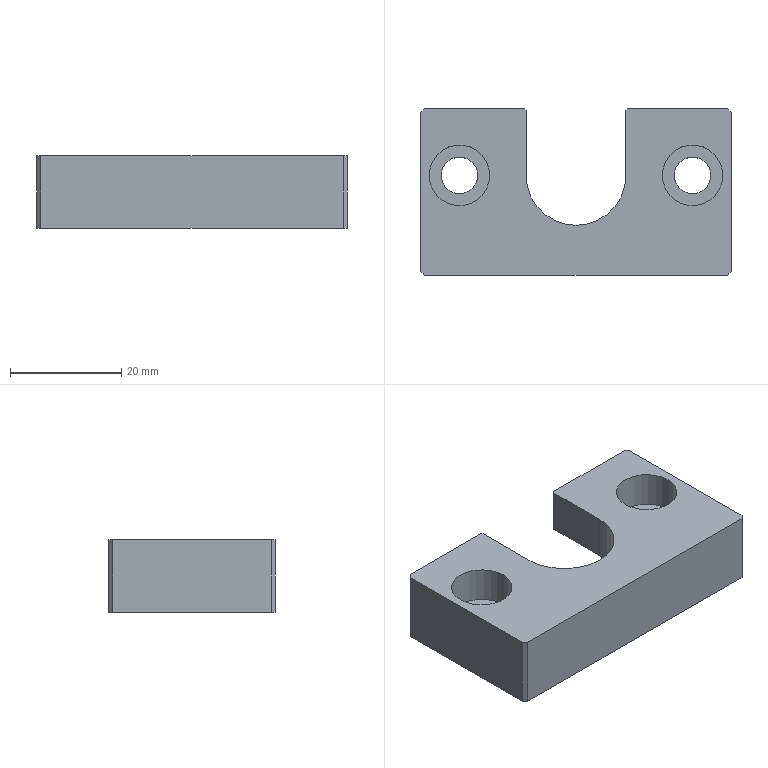Part | STEP file | HLRA16-a_2 | 1 solid | 30 faces | box 56 x 30 x 13 mm | volume 14203 mm3 | plane 20 | cylinder 10 | commonest cylinder face diameters 6.6 x4 10.9 x4 18 x1 28 x1